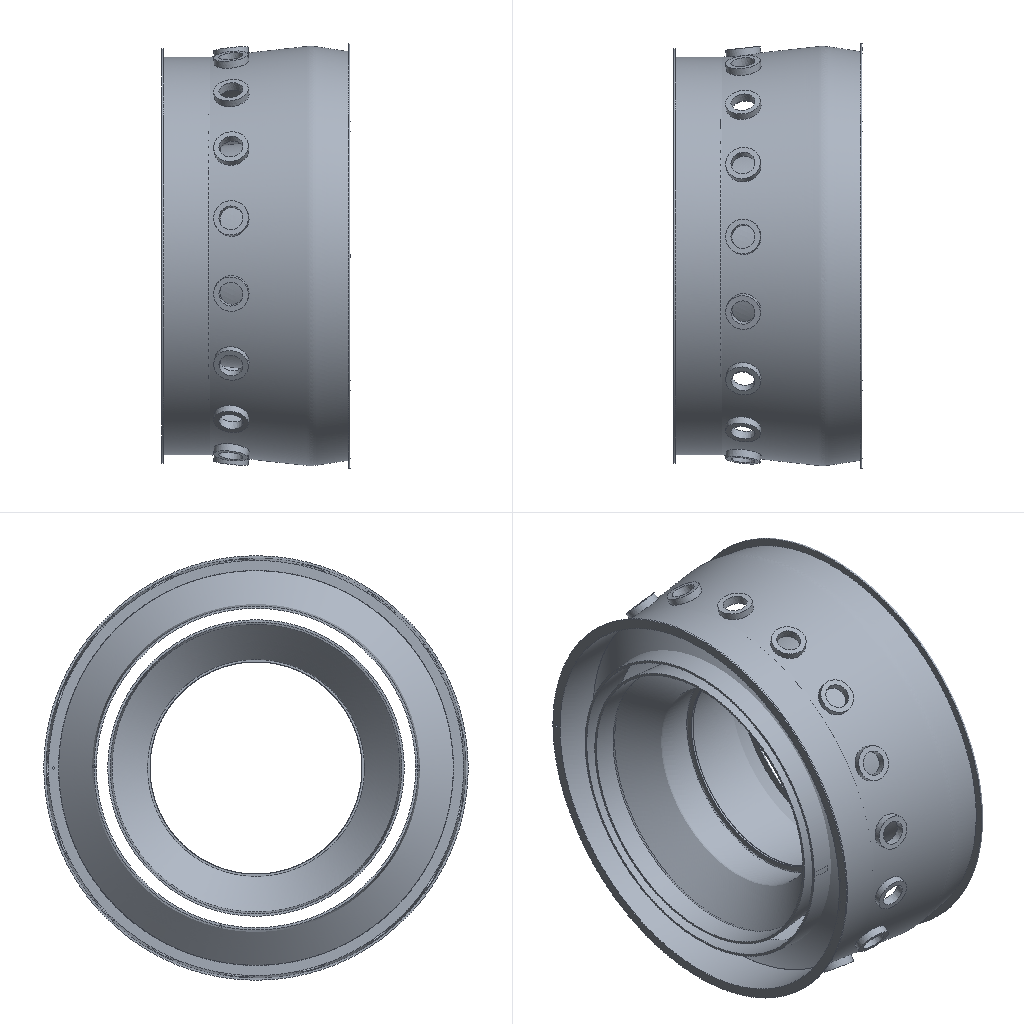Simulation study | ansys workbench
Set-up summary:
category,name,step,type,value,unit,region
solver,ansys_workbench
units,mm-N-s-tonne (MPa),,stated,"/units,MPA"
analysis,LS1,,static
load_step,LS1,LS1,static,nsubst=1; time=1
mesh,nodes,,,1043880
mesh,elements,,,774943
element_type,SOLID187,,,508745
element_type,SURF154,,,250330
element_type,CONTA174,,,7036
element_type,SOLID186,,,6528
element_type,TARGE170,,,2304
material,GH141,,E,216000
material,GH141,,nu,0.31
material,GH141,,density,8.27e-09,tonne mm^-3
material,GH141,,conductivity,8.37
material,GH141,,cte,1.054e-05
load,Define Pressure Using Surface Effect Elements,LS1,pressure,0.2,,SURF154 #16
load,Define Pressure Using Surface Effect Elements,LS1,pressure,0.25,,SURF154 #17
load,Define Pressure Using Surface Effect Elements,LS1,pressure,3.6,,SURF154 #18
load,,LS1,moment,"1e+08 [dir=(1, 0, 0) n=6]",,all
load,,LS1,force,"42000 [dir=(1, 0, 0) n=6]",,all
bc,Fixed Supports,model,fixed,[dofs=ALL],,_FIXEDSU
contact,Contact Region,,bonded (always),element=CONTA174
contact,contact 2,,bonded (always),element=CONTA174
contact,contact 3,,bonded (always),element=CONTA174
contact,contact 4,,bonded (always),element=CONTA174
contact,contact 5,,bonded (always),element=CONTA174
named_set,_FIXEDSU,,node,6895
Ansys APDL input file, long lists of numbers shortened:
/batch
/config,noeldb,1     ! force off writing results to database
*get,_wallstrt,active,,time,wall
! ANSYS input file written by Workbench version 2021 R1
! File used for geometry attach:
/title,____+__+__--____ (C5)
! ****** Begin Custom Load Command Snippet ******
/COM, ACT Extensions:
/COM,     LSDYNA, 2021.1
/COM,
! ****** End   Custom Load Command Snippet ******
*DIM,_wb_ProjectScratch_dir,string,248
_wb_ProjectScratch_dir(1) = ''
*DIM,_wb_SolverFiles_dir,string,248
_wb_SolverFiles_dir(1) = ''
*DIM,_wb_userfiles_dir,string,248
_wb_userfiles_dir(1) = ''
/com,--- Data in consistent NMM units. See Solving Units in the help system for more information.
/units,MPA
/nopr
/wb,file,start              !  signify a WB generated input file
/prep7
! Turn off shape checking because checks already performed inside WB mesher.
! See help system for more information.
SHPP,OFF,,NOWARN
/nolist
etcon,set             ! allow ANSYS to choose best KEYOP's for 180x elements, resets any applicable keyopt to MAPDL defaults
/com,*********** Nodes for the whole assembly ***********
nblock,3,,1148263
(1i9,3e20.9e3)
        1    -2.909328663E+02    -6.564341511E+00     4.578700000E+02
! (1043875 more lines like these left out)
-1
/com,*********** Nodes for all Remote Points ***********
nblock,3
(1i9,3e20.9e3)
  1043877    -7.493286614E+01    -6.564353799E+00     2.143080415E+02
  1043878    -7.493286951E+01    -6.697121594E+00     2.143200000E+02
  1043879    -7.493286951E+01    -6.697121594E+00     2.143200000E+02
  1043880    -7.493286580E+01    -6.533767534E+00     2.143199692E+02
-1
/wb,elem,start            !  set before creation of elements
/com,*********** Elements for Body 1 "____9.24_\____9.24_" ***********
et,1,187
eblock,19,solid,,320859
(19i9)
        1        1        1        1        0        0        0        0       10        0   194415   420982   429274   496877   520848   545299   607590   545303   545309
! (641717 more lines like these left out)
-1
/com,*********** Elements for Body 2 "____0923_ (1)-0\____0923_ (1)" ***********
et,2,186
keyo,2,2,1          ! set full integration on SOLID186
eblock,19,solid,,6528
(19i9)
        2        2        2        2        0        0        0        0       20        0        1     1050     1051    13262    13261     7008     7007    13469    13470
! (13055 more lines like these left out)
-1
/com,*********** Elements for Body 3 "______9.22_\______9.22_" ***********
et,3,187
eblock,19,solid,,92984
(19i9)
        3        3        3        3        0        0        0        0       10        0    35420    54545   103924   108327   107989   161558   401449   161564   161563
! (185967 more lines like these left out)
-1
/com,*********** Elements for Body 4 "______9.24_\______9.24_" ***********
et,4,187
eblock,19,solid,,66011
(19i9)
        4        4        3        4        0        0        0        0       10        0   128404    55040   108946   103353   108755   164427   399349   164424   164426
! (132021 more lines like these left out)
-1
/com,*********** Elements for Body 5 "____0923_ (1)\____0923_ (1)" ***********
et,5,187
eblock,19,solid,,28891
(19i9)
        5        5        3        5        0        0        0        0       10        0     6529    48274    97425   107256    48526   115927   382662   115929   115926
! (57781 more lines like these left out)
-1
/wb,elem,end               !  done creating elements
/com,*********** Send User Defined Coordinate System(s) ***********
csys,0
toffst,273.15,  ! Temperature offset from absolute zero
/com,*********** Set Reference Temperature ***********
tref,22.
/wb,mat,start              !  starting to send materials
/com,*********** Send Materials ***********
Temperature = 'TEMP' ! Temperature
MP,DENS,1,8.27e-09,	! tonne mm^-3
MPTEMP,,,,,,,,
MPTEMP,1,100
MPTEMP,2,200
MPTEMP,3,300
MPTEMP,4,400
MPTEMP,5,500
MPTEMP,6,600
MPTEMP,7,700
MPTEMP,8,800
MPTEMP,9,900
MPDATA,EX,1, ,216000,210000,205000,200000,195000,188000,
MPDATA,EX,1, ,182000,175000,168000,	! tonne s^-2 mm^-1
MPTEMP,,,,,,,,
MPTEMP,,,,,,,,
MPTEMP,1,100
MPTEMP,2,200
MPTEMP,3,300
MPTEMP,4,400
MPTEMP,5,500
MPTEMP,6,600
MPTEMP,7,700
MPTEMP,8,800
MPTEMP,9,900
MPDATA,NUXY,1, ,0.31,0.31,0.31,0.31,0.31,0.31,
MPDATA,NUXY,1, ,0.31,0.31,0.31,
MPTEMP,,,,,,,,
MPTEMP,,,,,,,,
MPTEMP,1,100
MPTEMP,2,200
MPTEMP,3,300
MPTEMP,4,400
MPTEMP,5,500
MPTEMP,6,600
MPTEMP,7,700
MPTEMP,8,800
MPTEMP,9,900
MPDATA,ALPX,1, ,1.054e-05,1.169e-05,1.224e-05,1.278e-05,1.308e-05,1.348e-05,
MPDATA,ALPX,1, ,1.421e-05,1.497e-05,1.591e-05,	! C^-1
MPTEMP,,,,,,,,
MPTEMP,,,,,,,,
MPTEMP,1,100
MPTEMP,2,200
MPTEMP,3,300
MPTEMP,4,400
MPTEMP,5,500
MPTEMP,6,600
MPTEMP,7,700
MPTEMP,8,800
MPTEMP,9,900
MPDATA,KXX,1, ,8.37,10.47,12.56,15.07,17.17,19.56,
MPDATA,KXX,1, ,21.35,23.45,25.96,	! tonne mm s^-3 C^-1
MPTEMP,,,,,,,,
Temperature = 'TEMP' ! Temperature
MP,DENS,2,8.27e-09,	! tonne mm^-3
MPTEMP,,,,,,,,
MPTEMP,1,100
MPTEMP,2,200
MPTEMP,3,300
MPTEMP,4,400
MPTEMP,5,500
MPTEMP,6,600
MPTEMP,7,700
MPTEMP,8,800
MPTEMP,9,900
MPDATA,EX,2, ,216000,210000,205000,200000,195000,188000,
MPDATA,EX,2, ,182000,175000,168000,	! tonne s^-2 mm^-1
MPTEMP,,,,,,,,
MPTEMP,,,,,,,,
MPTEMP,1,100
MPTEMP,2,200
MPTEMP,3,300
MPTEMP,4,400
MPTEMP,5,500
MPTEMP,6,600
MPTEMP,7,700
MPTEMP,8,800
MPTEMP,9,900
MPDATA,NUXY,2, ,0.31,0.31,0.31,0.31,0.31,0.31,
MPDATA,NUXY,2, ,0.31,0.31,0.31,
MPTEMP,,,,,,,,
MPTEMP,,,,,,,,
MPTEMP,1,100
MPTEMP,2,200
MPTEMP,3,300
MPTEMP,4,400
MPTEMP,5,500
MPTEMP,6,600
MPTEMP,7,700
MPTEMP,8,800
MPTEMP,9,900
MPDATA,ALPX,2, ,1.054e-05,1.169e-05,1.224e-05,1.278e-05,1.308e-05,1.348e-05,
MPDATA,ALPX,2, ,1.421e-05,1.497e-05,1.591e-05,	! C^-1
MPTEMP,,,,,,,,
MPTEMP,,,,,,,,
MPTEMP,1,100
MPTEMP,2,200
MPTEMP,3,300
MPTEMP,4,400
MPTEMP,5,500
MPTEMP,6,600
MPTEMP,7,700
MPTEMP,8,800
MPTEMP,9,900
MPDATA,KXX,2, ,8.37,10.47,12.56,15.07,17.17,19.56,
MPDATA,KXX,2, ,21.35,23.45,25.96,	! tonne mm s^-3 C^-1
MPTEMP,,,,,,,,
Temperature = 'TEMP' ! Temperature
MP,DENS,3,8.27e-09,	! tonne mm^-3
MPTEMP,,,,,,,,
MPTEMP,1,100
MPTEMP,2,200
MPTEMP,3,300
MPTEMP,4,400
MPTEMP,5,500
MPTEMP,6,600
MPTEMP,7,700
MPTEMP,8,800
MPTEMP,9,900
MPDATA,EX,3, ,216000,210000,205000,200000,195000,188000,
MPDATA,EX,3, ,182000,175000,168000,	! tonne s^-2 mm^-1
MPTEMP,,,,,,,,
MPTEMP,,,,,,,,
MPTEMP,1,100
MPTEMP,2,200
MPTEMP,3,300
MPTEMP,4,400
MPTEMP,5,500
MPTEMP,6,600
MPTEMP,7,700
MPTEMP,8,800
MPTEMP,9,900
MPDATA,NUXY,3, ,0.31,0.31,0.31,0.31,0.31,0.31,
MPDATA,NUXY,3, ,0.31,0.31,0.31,
MPTEMP,,,,,,,,
MPTEMP,,,,,,,,
MPTEMP,1,100
MPTEMP,2,200
MPTEMP,3,300
MPTEMP,4,400
MPTEMP,5,500
MPTEMP,6,600
MPTEMP,7,700
MPTEMP,8,800
MPTEMP,9,900
MPDATA,ALPX,3, ,1.054e-05,1.169e-05,1.224e-05,1.278e-05,1.308e-05,1.348e-05,
MPDATA,ALPX,3, ,1.421e-05,1.497e-05,1.591e-05,	! C^-1
MPTEMP,,,,,,,,
MPTEMP,,,,,,,,
MPTEMP,1,100
MPTEMP,2,200
MPTEMP,3,300
MPTEMP,4,400
MPTEMP,5,500
MPTEMP,6,600
MPTEMP,7,700
MPTEMP,8,800
MPTEMP,9,900
MPDATA,KXX,3, ,8.37,10.47,12.56,15.07,17.17,19.56,
MPDATA,KXX,3, ,21.35,23.45,25.96,	! tonne mm s^-3 C^-1
MPTEMP,,,,,,,,
Temperature = 'TEMP' ! Temperature
MP,DENS,4,8.27e-09,	! tonne mm^-3
MPTEMP,,,,,,,,
MPTEMP,1,100
MPTEMP,2,200
MPTEMP,3,300
MPTEMP,4,400
MPTEMP,5,500
MPTEMP,6,600
MPTEMP,7,700
MPTEMP,8,800
MPTEMP,9,900
MPDATA,EX,4, ,216000,210000,205000,200000,195000,188000,
MPDATA,EX,4, ,182000,175000,168000,	! tonne s^-2 mm^-1
MPTEMP,,,,,,,,
MPTEMP,,,,,,,,
MPTEMP,1,100
MPTEMP,2,200
MPTEMP,3,300
MPTEMP,4,400
MPTEMP,5,500
MPTEMP,6,600
MPTEMP,7,700
MPTEMP,8,800
MPTEMP,9,900
MPDATA,NUXY,4, ,0.31,0.31,0.31,0.31,0.31,0.31,
MPDATA,NUXY,4, ,0.31,0.31,0.31,
MPTEMP,,,,,,,,
MPTEMP,,,,,,,,
MPTEMP,1,100
MPTEMP,2,200
MPTEMP,3,300
MPTEMP,4,400
MPTEMP,5,500
MPTEMP,6,600
MPTEMP,7,700
MPTEMP,8,800
MPTEMP,9,900
MPDATA,ALPX,4, ,1.054e-05,1.169e-05,1.224e-05,1.278e-05,1.308e-05,1.348e-05,
MPDATA,ALPX,4, ,1.421e-05,1.497e-05,1.591e-05,	! C^-1
MPTEMP,,,,,,,,
MPTEMP,,,,,,,,
MPTEMP,1,100
MPTEMP,2,200
MPTEMP,3,300
MPTEMP,4,400
MPTEMP,5,500
MPTEMP,6,600
MPTEMP,7,700
MPTEMP,8,800
MPTEMP,9,900
MPDATA,KXX,4, ,8.37,10.47,12.56,15.07,17.17,19.56,
MPDATA,KXX,4, ,21.35,23.45,25.96,	! tonne mm s^-3 C^-1
MPTEMP,,,,,,,,
Temperature = 'TEMP' ! Temperature
MP,DENS,5,8.27e-09,	! tonne mm^-3
MPTEMP,,,,,,,,
MPTEMP,1,100
MPTEMP,2,200
MPTEMP,3,300
MPTEMP,4,400
MPTEMP,5,500
MPTEMP,6,600
MPTEMP,7,700
MPTEMP,8,800
MPTEMP,9,900
MPDATA,EX,5, ,216000,210000,205000,200000,195000,188000,
MPDATA,EX,5, ,182000,175000,168000,	! tonne s^-2 mm^-1
MPTEMP,,,,,,,,
MPTEMP,,,,,,,,
MPTEMP,1,100
MPTEMP,2,200
MPTEMP,3,300
MPTEMP,4,400
MPTEMP,5,500
MPTEMP,6,600
MPTEMP,7,700
MPTEMP,8,800
MPTEMP,9,900
MPDATA,NUXY,5, ,0.31,0.31,0.31,0.31,0.31,0.31,
MPDATA,NUXY,5, ,0.31,0.31,0.31,
MPTEMP,,,,,,,,
MPTEMP,,,,,,,,
MPTEMP,1,100
MPTEMP,2,200
MPTEMP,3,300
MPTEMP,4,400
MPTEMP,5,500
MPTEMP,6,600
MPTEMP,7,700
MPTEMP,8,800
MPTEMP,9,900
MPDATA,ALPX,5, ,1.054e-05,1.169e-05,1.224e-05,1.278e-05,1.308e-05,1.348e-05,
MPDATA,ALPX,5, ,1.421e-05,1.497e-05,1.591e-05,	! C^-1
MPTEMP,,,,,,,,
MPTEMP,,,,,,,,
MPTEMP,1,100
MPTEMP,2,200
MPTEMP,3,300
MPTEMP,4,400
MPTEMP,5,500
MPTEMP,6,600
MPTEMP,7,700
MPTEMP,8,800
MPTEMP,9,900
MPDATA,KXX,5, ,8.37,10.47,12.56,15.07,17.17,19.56,
MPDATA,KXX,5, ,21.35,23.45,25.96,	! tonne mm s^-3 C^-1
MPTEMP,,,,,,,,
/wb,mat,end                !  done sending materials
!************************* Model Summary ********************
!____9.24_\____9.24_,	GH141,	matid,	1
!____0923_ (1)-0\____0923_ (1),	GH141,	matid,	2
!______9.22_\______9.22_,	GH141,	matid,	3
!______9.24_\______9.24_,	GH141,	matid,	4
!____0923_ (1)\____0923_ (1),	GH141,	matid,	5
!************************* End Model Summary ********************
! get the diagonal of the bounding box. Needed later for other things
*get,_xmin,node,,mnloc,x
*get,_ymin,node,,mnloc,y
*get,_zmin,node,,mnloc,z
*get,_xmax,node,,mxloc,x
*get,_ymax,node,,mxloc,y
*get,_zmax,node,,mxloc,z
_ASMDIAG=(_xmax-_xmin)*(_xmax-_xmin)+(_ymax-_ymin)*(_ymax-_ymin)+(_zmax-_zmin)*(_zmax-_zmin)
_ASMDIAG=SQRT(_ASMDIAG)
/wb,contact,start          !  starting to send contact
/com,*********** Create Contact "接触区域" ***********
/com,            Real Constant Set For Above Contact Is 7 & 6
*set,tid,7
*set,cid,6
r,tid
r,cid
et,tid,170
et,cid,174
eblock,10,,,768
(15i9)
   851574        7        7        7        0   423188   423189   423572   423572   564570   564576   423572   564572
! (767 more lines like these left out)
-1
eblock,10,,,768
(15i9)
   852342        6        6        6        0   423188   423189   423572   423572   564570   564576   423572   564572
! (767 more lines like these left out)
-1
eblock,10,,,1536
(15i9)
   853110        6        7        6        0     3446     3063     6901     6902    22949    22950    34083    24100
! (1535 more lines like these left out)
-1
eblock,10,,,1536
(15i9)
   854646        7        6        7        0     3446     3063     6901     6902    22949    22950    34083    24100
! (1535 more lines like these left out)
-1
keyo,cid,8,2               ! auto create asymmetric contact (from Program Controlled setting)
keyo,cid,10,0              ! adjust contact stiffness each NR iteration (from Program Controlled setting)
keyo,cid,12,5              ! bonded always
keyo,cid,18,1              ! small sliding turned on by application
keyo,cid,2,0               ! augmented Lagrange (from Program Controlled setting)
keyo,cid,4,0               ! on Gauss point (from Program Controlled setting)
keyo,cid,9,1               ! ignore initial gaps/penetration
keyo,cid,7,0               ! No Prediction
rmod,tid,3,10.      ! FKN
rmod,tid,5,0.       ! ICONT
rmod,tid,6,0.       ! PINB
rmod,tid,10,0.      ! CNOF
rmod,tid,12,0.      ! FKT
rmod,tid,36,113     ! WB DSID
rmod,cid,3,10.      ! FKN
rmod,cid,5,0.       ! ICONT
rmod,cid,6,0.       ! PINB
rmod,cid,10,0.      ! CNOF
rmod,cid,12,0.      ! FKT
rmod,cid,36,113     ! WB DSID
nsel,all
esel,all
/wb,contact,end            !  done creating contacts
/golist
/wb,load,start             !  starting to send loads
/com,*********** Fixed Supports ***********
CMBLOCK,_FIXEDSU,NODE,     6895
(8i10)
      6893      6894      6911      6912      6913      6914      6915      6916
! (861 more lines like these left out)
cmsel,s,_FIXEDSU
d,all,all
nsel,all
/com,*********** Create Remote Point "内部远程点" ***********
! -------- Remote Point Used by "外机匣扭矩" --------
*set,tid,9
*set,cid,8
et,cid,174
et,tid,170
keyo,tid,2,1               ! Don't fix the pilot node
keyo,tid,4,111111
keyo,cid,12,5              ! Bonded Contact
keyo,cid,4,1               ! Deformable RBE3 style load
keyo,cid,2,2               ! MPC style contact
eblock,10,,,1466
(15i9)
   856182        8        8        8        0   418454   418455   515807   515807   527672   527684   515807   527677
! (1465 more lines like these left out)
-1
*set,_npilot,1043879
_npilot146=_npilot
type,tid
mat ,cid
real,cid
tshape,pilo
en,857648,_npilot
tshape
/com,*********** Create Remote Point "内部远程点 2" ***********
! -------- Remote Point Used by "内机匣扭矩" --------
*set,tid,11
*set,cid,10
et,cid,174
et,tid,170
keyo,tid,2,1               ! Don't fix the pilot node
keyo,tid,4,111111
keyo,cid,12,5              ! Bonded Contact
keyo,cid,4,1               ! Deformable RBE3 style load
keyo,cid,2,2               ! MPC style contact
eblock,10,,,900
(15i9)
   857649       10       10       10        0    51746   106176    51747    51747   141736   141741    51747   141734
! (899 more lines like these left out)
-1
*set,_npilot,1043880
_npilot149=_npilot
type,tid
mat ,cid
real,cid
tshape,pilo
en,858549,_npilot
tshape
/com,*********** Create Remote Point "远程点" ***********
*set,tid,13
*set,cid,12
et,cid,174
et,tid,170
keyo,tid,2,1               ! Don't fix the pilot node
keyo,tid,4,111111
keyo,cid,12,5              ! Bonded Contact
keyo,cid,4,1               ! Deformable RBE3 style load
keyo,cid,2,2               ! MPC style contact
eblock,10,,,900
(15i9)
   858550       12       12       12        0    51746   106176    51747    51747   141736   141741    51747   141734
! (899 more lines like these left out)
-1
*set,_npilot,1043877
_npilot87=_npilot
type,tid
mat ,cid
real,cid
tshape,pilo
en,859450,_npilot
tshape
/com,*********** Create Remote Point "远程点 2" ***********
*set,tid,15
*set,cid,14
et,cid,174
et,tid,170
keyo,tid,2,1               ! Don't fix the pilot node
keyo,tid,4,111111
keyo,cid,12,5              ! Bonded Contact
keyo,cid,4,1               ! Deformable RBE3 style load
keyo,cid,2,2               ! MPC style contact
eblock,10,,,1466
(15i9)
   859451       14       14       14        0   418454   418455   515807   515807   527672   527684   515807   527677
! (1465 more lines like these left out)
-1
*set,_npilot,1043878
_npilot89=_npilot
type,tid
mat ,cid
real,cid
tshape,pilo
en,860917,_npilot
tshape
/com,*********** Define Pressure Using Surface Effect Elements ***********
et,16,154
eblock,10,,,54795
(15i9)
   860918       16       16       16        0    66408    66113    66706    66706   228927   228929    66706   230400
! (54794 more lines like these left out)
-1
esel,s,type,,16
keyop,16,7,0                ! Use deformed area for application of load
esel,all
/com,*********** Define Pressure Using Surface Effect Elements ***********
et,17,154
eblock,10,,,99919
(15i9)
   915713       17       17       17        0   471984   472470   472955   472955   832353   833495   472955   832354
! (99918 more lines like these left out)
-1
esel,s,type,,17
keyop,17,7,0                ! Use deformed area for application of load
esel,all
/com,*********** Define Pressure Using Surface Effect Elements ***********
et,18,154
eblock,10,,,95616
(15i9)
  1015632       18       18       18        0    73498    73497    73900    73900   278870   278872    73900   278874
! (95615 more lines like these left out)
-1
esel,s,type,,18
keyop,18,7,0                ! Use deformed area for application of load
esel,all
/com,*********** Construct Moment Using Remote Attachment ***********
*DIM,_loadvari145x,TABLE,2,1,1,TIME,
! Time values
_loadvari145x(1,0,1) = 0.
_loadvari145x(2,0,1) = 1.
! Load values
_loadvari145x(1,1,1) = 0.
_loadvari145x(2,1,1) = 50000000.
*DIM,_loadvari145y,TABLE,2,1,1,TIME,
! Time values
_loadvari145y(1,0,1) = 0.
_loadvari145y(2,0,1) = 1.
! Load values
_loadvari145y(1,1,1) = 0.
_loadvari145y(2,1,1) = 0.
*DIM,_loadvari145z,TABLE,2,1,1,TIME,
! Time values
_loadvari145z(1,0,1) = 0.
_loadvari145z(2,0,1) = 1.
! Load values
_loadvari145z(1,1,1) = 0.
_loadvari145z(2,1,1) = 0.
/com,*********** Construct Moment Using Remote Attachment ***********
*DIM,_loadvari148x,TABLE,2,1,1,TIME,
! Time values
_loadvari148x(1,0,1) = 0.
_loadvari148x(2,0,1) = 1.
! Load values
_loadvari148x(1,1,1) = 0.
_loadvari148x(2,1,1) = 50000000.
*DIM,_loadvari148y,TABLE,2,1,1,TIME,
! Time values
_loadvari148y(1,0,1) = 0.
_loadvari148y(2,0,1) = 1.
! Load values
_loadvari148y(1,1,1) = 0.
_loadvari148y(2,1,1) = 0.
*DIM,_loadvari148z,TABLE,2,1,1,TIME,
! Time values
_loadvari148z(1,0,1) = 0.
_loadvari148z(2,0,1) = 1.
! Load values
_loadvari148z(1,1,1) = 0.
_loadvari148z(2,1,1) = 0.
/com,*********** Construct Remote Force ***********
*DIM,_loadvari151x,TABLE,2,1,1,TIME,
! Time values
_loadvari151x(1,0,1) = 0.
_loadvari151x(2,0,1) = 1.
! Load values
_loadvari151x(1,1,1) = 0.
_loadvari151x(2,1,1) = 21000.
*DIM,_loadvari151y,TABLE,2,1,1,TIME,
! Time values
_loadvari151y(1,0,1) = 0.
_loadvari151y(2,0,1) = 1.
! Load values
_loadvari151y(1,1,1) = 0.
_loadvari151y(2,1,1) = 0.
*DIM,_loadvari151z,TABLE,2,1,1,TIME,
! Time values
_loadvari151z(1,0,1) = 0.
_loadvari151z(2,0,1) = 1.
! Load values
_loadvari151z(1,1,1) = 0.
_loadvari151z(2,1,1) = 0.
/com,*********** Construct Remote Force ***********
*DIM,_loadvari153x,TABLE,2,1,1,TIME,
! Time values
_loadvari153x(1,0,1) = 0.
_loadvari153x(2,0,1) = 1.
! Load values
_loadvari153x(1,1,1) = 0.
_loadvari153x(2,1,1) = 21000.
*DIM,_loadvari153y,TABLE,2,1,1,TIME,
! Time values
_loadvari153y(1,0,1) = 0.
_loadvari153y(2,0,1) = 1.
! Load values
_loadvari153y(1,1,1) = 0.
_loadvari153y(2,1,1) = 0.
*DIM,_loadvari153z,TABLE,2,1,1,TIME,
! Time values
_loadvari153z(1,0,1) = 0.
_loadvari153z(2,0,1) = 1.
! Load values
_loadvari153z(1,1,1) = 0.
_loadvari153z(2,1,1) = 0.
esel,all
/gst,on,on
fini
*get,_numnode,node,0,count
*get,_numelem,elem,0,count
*get, _MAXELEMNUM, elem, 0, NUM, MAX
*get, _MAXNODENUM, node, 0, NUM, MAX
*get, _MAXELEMTYPE, etyp, 0, NUM, MAX
*get, _MAXREALCONST, real, 0, NUM, MAX
/go
/wb,load,end               !  done creating loads
/com,--- Number of total nodes = %_numnode%
/com,--- Number of contact elements = 259670
/com,--- Number of spring elements = 0
/com,--- Number of bearing elements = 0
/com,--- Number of solid elements = 515273
/com,--- Number of condensed parts = 0
/com,--- Number of total elements = %_numelem%
*get,_wallbsol,active,,time,wall
/com,****************************************************************************
/com,*************************    SOLUTION       ********************************
/com,****************************************************************************
/solu
antype,0                   ! static analysis
_thickRatio=  0     ! Ratio of thick parts in the model
eqsl,sparse,,,,,1
cntr,print,1               ! print out contact info and also make no initial contact an error
dmpoption,emat,no             ! Don't combine emat file for DANSYS
dmpoption,esav,no             ! Don't combine esav file for DANSYS
nldiag,cont,iter           ! print out contact info each equilibrium iteration
rescontrol,,none                 ! Do not keep any restart files
/com,****************************************************
/com,******************* SOLVE FOR LS 1 OF 1 ****************
esel,s,type,,16
nsle
sf,all,pres,0.2
esel,s,type,,17
nsle
sf,all,pres,0.25
esel,s,type,,18
nsle
sf,all,pres,3.6
nsel,all
esel,all
nsel,s,node,,1043879
f,all,mx,%_loadvari145x%
f,all,my,%_loadvari145y%
f,all,mz,%_loadvari145z%
nsel,s,node,,1043880
f,all,mx,%_loadvari148x%
f,all,my,%_loadvari148y%
f,all,mz,%_loadvari148z%
nsel,all
nsel,s,node,,1043878
f,all,fx,%_loadvari151x%
f,all,fy,%_loadvari151y%
f,all,fz,%_loadvari151z%
nsel,s,node,,1043877
f,all,fx,%_loadvari153x%
f,all,fy,%_loadvari153y%
f,all,fz,%_loadvari153z%
nsel,all
esel,all
/nopr
/gopr
/nolist
nsub,1,1,1
time,1.
outres,erase
outres,all,none
outres,nsol,all,
outres,rsol,all
outres,eangl,all
outres,etmp,all
outres,veng,all
outres,strs,all,
outres,epel,all,
outres,eppl,all,
outres,cont,all,
! *********** WB SOLVE COMMAND ***********
! check interactive state
*get,ANSINTER_,active,,int
*if,ANSINTER_,ne,0,then
/eof
*endif
solve
/com *************** Write FE CONNECTORS *********
CEWRITE,file,ce,,INTE
/com,****************************************************
/com,*************** FINISHED SOLVE FOR LS 1 *************
*get,_wallasol,active,,time,wall
/nopr
*get,_numnode,node,0,count
*get,_numelem,elem,0,count
*get, _MAXELEMNUM, elem, 0, NUM, MAX
*get, _MAXNODENUM, node, 0, NUM, MAX,,,INTERNAL
*get, _MAXELEMTYPE, etyp, 0, NUM, MAX
*get, _MAXREALCONST, real, 0, NUM, MAX
/gopr
/post1
xmlo,ENCODING,ISO-8859-1
xmlo,parm
/xml,parm,xml
fini
/gopr
*get,_walldone,active,,time,wall
_preptime=(_wallbsol-_wallstrt)*3600
_solvtime=(_wallasol-_wallbsol)*3600
_posttime=(_walldone-_wallasol)*3600
_totaltim=(_walldone-_wallstrt)*3600
*get,_dlbratio,active,0,solu,dlbr
*get,_combtime,active,0,solu,comb
/com,--- Total number of nodes = %_numnode%
/com,--- Total number of elements = %_numelem%
/com,--- Element load balance ratio = %_dlbratio%
/com,--- Time to combine distributed files = %_combtime%
/wb,file,end               ! done with WB generated input
Results summary:
result,analyses[0].index,,,1
result,analyses[0].system,,,SYS-2
result,analyses[0].deck,,,deck.dat
result,analyses[0].solve_status,,,completed
result,analyses[0].analysis_type,,,static
result,analyses[0].physics,,,mechanical
result,analyses[0].unit_system,,,"NMM: mm, ton, N, s, mV, mA, degC"
result,analyses[0].n_sets,,,1
result,analyses[0].load_steps[0].set,set=1,,1
result,analyses[0].load_steps[0].time_or_freq,set=1,,1
result,analyses[0].load_steps[0].max_displacement_magnitude,set=1,,0.8079
result,analyses[0].load_steps[0].max_von_mises_nodal,set=1,,1059.21
result,analyses[0].load_steps[0].reaction_force_sum_xyz[1],set=1,,405553
result,analyses[0].load_steps[0].reaction_force_sum_xyz[2],set=1,,-0.0004945
result,analyses[0].load_steps[0].reaction_force_sum_xyz[3],set=1,,-0.0006192
result,geometry_export[0][0],,,1.step
result,geometry_export[0][1],,,ok
result,geometry_export[0][2],,,39
result,geometry_export[1][0],,,2.step
result,geometry_export[1][1],,,ok
result,geometry_export[1][2],,,5